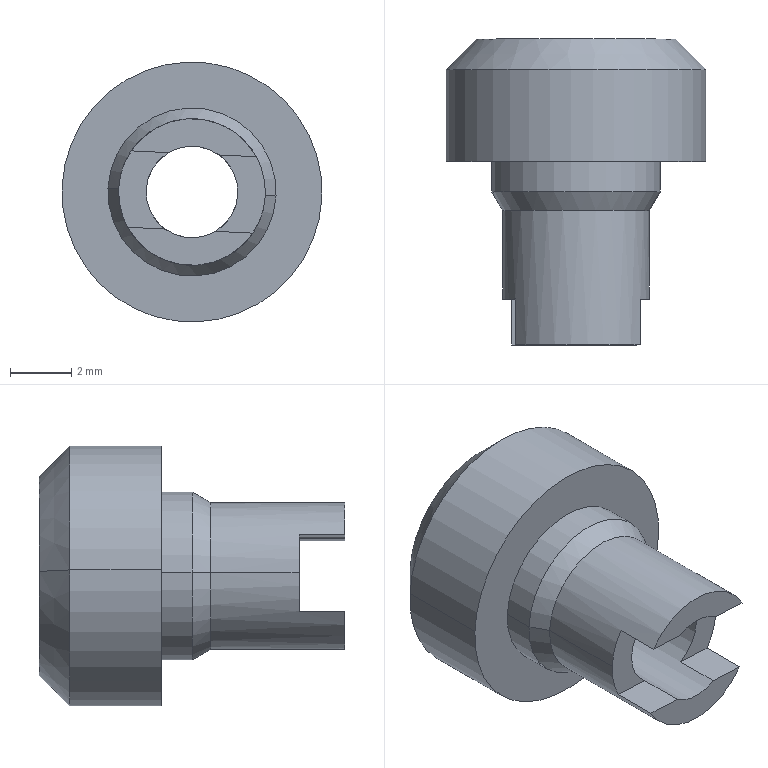Part | SolidWorks | features BaseBody 1 | 1 solid | 24 faces | box 8.5 x 10 x 8.5 mm | volume 252.316 mm3 | plane 10 | cylinder 8 | cone 6 | commonest cylinder face diameters 3 x2 4.8 x2 5.5 x2 8.5 x2
STEP:
#1=CARTESIAN_POINT('',(230.998,190.9,-0.07029));
#2=VERTEX_POINT('',#1);
#3=CARTESIAN_POINT('',(228.002,190.9,0.07029));
#4=VERTEX_POINT('',#3);
#5=CARTESIAN_POINT('',(229.5,190.9,0.));
#6=DIRECTION('',(0.,1.,0.));
#7=DIRECTION('',(0.9989,0.,-0.04686));
#8=AXIS2_PLACEMENT_3D('',#5,#6,#7);
#9=CIRCLE('',#8,1.5);
#10=EDGE_CURVE('',#2,#4,#9,.T.);
#11=ORIENTED_EDGE('',*,*,#10,.F.);
#12=CARTESIAN_POINT('',(231.198,191.1,-0.07966));
#13=VERTEX_POINT('',#12);
#14=CARTESIAN_POINT('',(230.998,190.9,-0.07029));
#15=DIRECTION('',(0.7063,0.7071,-0.03314));
#16=VECTOR('',#15,1000.);
#17=LINE('',#14,#16);
#18=EDGE_CURVE('',#2,#13,#17,.T.);
#19=ORIENTED_EDGE('',*,*,#18,.T.);
#20=CARTESIAN_POINT('',(227.802,191.1,0.07966));
#21=VERTEX_POINT('',#20);
#22=CARTESIAN_POINT('',(229.5,191.1,0.));
#23=DIRECTION('',(0.,-1.,0.));
#24=DIRECTION('',(0.9989,0.,-0.04686));
#25=AXIS2_PLACEMENT_3D('',#22,#23,#24);
#26=CIRCLE('',#25,1.7);
#27=EDGE_CURVE('',#21,#13,#26,.T.);
#28=ORIENTED_EDGE('',*,*,#27,.F.);
#29=CARTESIAN_POINT('',(228.002,190.9,0.07029));
#30=DIRECTION('',(-0.7063,0.7071,0.03314));
#31=VECTOR('',#30,1000.);
#32=LINE('',#29,#31);
#33=EDGE_CURVE('',#4,#21,#32,.T.);
#34=ORIENTED_EDGE('',*,*,#33,.F.);
#35=EDGE_LOOP('',(#11,#19,#28,#34));
#36=FACE_OUTER_BOUND('',#35,.T.);
#37=CARTESIAN_POINT('',(229.5,190.9,0.));
#38=DIRECTION('',(0.,1.,0.));
#39=DIRECTION('',(-0.9989,0.,0.04686));
#40=AXIS2_PLACEMENT_3D('',#37,#38,#39);
#41=CONICAL_SURFACE('',#40,1.5,0.7854);
#42=ADVANCED_FACE('',(#36),#41,.F.);
#43=CARTESIAN_POINT('',(226.254,191.1,0.1523));
#44=VERTEX_POINT('',#43);
#45=CARTESIAN_POINT('',(232.746,191.1,-0.1523));
#46=VERTEX_POINT('',#45);
#47=CARTESIAN_POINT('',(229.5,191.1,0.));
#48=DIRECTION('',(0.,1.,0.));
#49=DIRECTION('',(0.9989,0.,-0.04686));
#50=AXIS2_PLACEMENT_3D('',#47,#48,#49);
#51=CIRCLE('',#50,3.25);
#52=EDGE_CURVE('',#44,#46,#51,.T.);
#53=ORIENTED_EDGE('',*,*,#52,.F.);
#54=CARTESIAN_POINT('',(225.255,190.1,0.1992));
#55=VERTEX_POINT('',#54);
#56=CARTESIAN_POINT('',(226.254,191.1,0.1523));
#57=DIRECTION('',(-0.7063,-0.7071,0.03314));
#58=VECTOR('',#57,1000.);
#59=LINE('',#56,#58);
#60=EDGE_CURVE('',#44,#55,#59,.T.);
#61=ORIENTED_EDGE('',*,*,#60,.T.);
#62=CARTESIAN_POINT('',(233.745,190.1,-0.1992));
#63=VERTEX_POINT('',#62);
#64=CARTESIAN_POINT('',(229.5,190.1,0.));
#65=DIRECTION('',(0.,-1.,0.));
#66=DIRECTION('',(0.9989,0.,-0.04686));
#67=AXIS2_PLACEMENT_3D('',#64,#65,#66);
#68=CIRCLE('',#67,4.25);
#69=EDGE_CURVE('',#63,#55,#68,.T.);
#70=ORIENTED_EDGE('',*,*,#69,.F.);
#71=CARTESIAN_POINT('',(232.746,191.1,-0.1523));
#72=DIRECTION('',(0.7063,-0.7071,-0.03314));
#73=VECTOR('',#72,1000.);
#74=LINE('',#71,#73);
#75=EDGE_CURVE('',#46,#63,#74,.T.);
#76=ORIENTED_EDGE('',*,*,#75,.F.);
#77=EDGE_LOOP('',(#53,#61,#70,#76));
#78=FACE_OUTER_BOUND('',#77,.T.);
#79=CARTESIAN_POINT('',(229.5,191.1,0.));
#80=DIRECTION('',(0.,-1.,0.));
#81=DIRECTION('',(0.9989,0.,-0.04686));
#82=AXIS2_PLACEMENT_3D('',#79,#80,#81);
#83=CONICAL_SURFACE('',#82,3.25,0.7854);
#84=ADVANCED_FACE('',(#78),#83,.T.);
#85=CARTESIAN_POINT('',(227.103,185.494,0.1125));
#86=VERTEX_POINT('',#85);
#87=CARTESIAN_POINT('',(231.897,185.494,-0.1125));
#88=VERTEX_POINT('',#87);
#89=CARTESIAN_POINT('',(229.5,185.494,0.));
#90=DIRECTION('',(0.,1.,0.));
#91=DIRECTION('',(-0.9989,0.,0.04686));
#92=AXIS2_PLACEMENT_3D('',#89,#90,#91);
#93=CIRCLE('',#92,2.4);
#94=EDGE_CURVE('',#86,#88,#93,.T.);
#95=ORIENTED_EDGE('',*,*,#94,.T.);
#96=CARTESIAN_POINT('',(232.247,186.1,-0.1289));
#97=VERTEX_POINT('',#96);
#98=CARTESIAN_POINT('',(231.897,185.494,-0.1125));
#99=DIRECTION('',(0.4995,0.866,-0.02343));
#100=VECTOR('',#99,1000.);
#101=LINE('',#98,#100);
#102=EDGE_CURVE('',#88,#97,#101,.T.);
#103=ORIENTED_EDGE('',*,*,#102,.T.);
#104=CARTESIAN_POINT('',(226.753,186.1,0.1289));
#105=VERTEX_POINT('',#104);
#106=CARTESIAN_POINT('',(229.5,186.1,0.));
#107=DIRECTION('',(0.,1.,0.));
#108=DIRECTION('',(-0.9989,0.,0.04686));
#109=AXIS2_PLACEMENT_3D('',#106,#107,#108);
#110=CIRCLE('',#109,2.75);
#111=EDGE_CURVE('',#105,#97,#110,.T.);
#112=ORIENTED_EDGE('',*,*,#111,.F.);
#113=CARTESIAN_POINT('',(227.103,185.494,0.1125));
#114=DIRECTION('',(-0.4995,0.866,0.02343));
#115=VECTOR('',#114,1000.);
#116=LINE('',#113,#115);
#117=EDGE_CURVE('',#86,#105,#116,.T.);
#118=ORIENTED_EDGE('',*,*,#117,.F.);
#119=EDGE_LOOP('',(#95,#103,#112,#118));
#120=FACE_OUTER_BOUND('',#119,.T.);
#121=CARTESIAN_POINT('',(229.5,185.494,0.));
#122=DIRECTION('',(0.,1.,0.));
#123=DIRECTION('',(-0.9989,0.,0.04686));
#124=AXIS2_PLACEMENT_3D('',#121,#122,#123);
#125=CONICAL_SURFACE('',#124,2.4,0.5236);
#126=ADVANCED_FACE('',(#120),#125,.T.);
#127=ORIENTED_EDGE('',*,*,#111,.T.);
#128=CARTESIAN_POINT('',(232.247,187.1,-0.1289));
#129=VERTEX_POINT('',#128);
#130=CARTESIAN_POINT('',(232.247,192.536,-0.1289));
#131=DIRECTION('',(0.,1.,0.));
#132=VECTOR('',#131,1000.);
#133=LINE('',#130,#132);
#134=EDGE_CURVE('',#97,#129,#133,.T.);
#135=ORIENTED_EDGE('',*,*,#134,.T.);
#136=CARTESIAN_POINT('',(226.753,187.1,0.1289));
#137=VERTEX_POINT('',#136);
#138=CARTESIAN_POINT('',(229.5,187.1,0.));
#139=DIRECTION('',(0.,1.,0.));
#140=DIRECTION('',(-0.9989,0.,0.04686));
#141=AXIS2_PLACEMENT_3D('',#138,#139,#140);
#142=CIRCLE('',#141,2.75);
#143=EDGE_CURVE('',#137,#129,#142,.T.);
#144=ORIENTED_EDGE('',*,*,#143,.F.);
#145=CARTESIAN_POINT('',(226.753,192.536,0.1289));
#146=DIRECTION('',(0.,1.,0.));
#147=VECTOR('',#146,1000.);
#148=LINE('',#145,#147);
#149=EDGE_CURVE('',#105,#137,#148,.T.);
#150=ORIENTED_EDGE('',*,*,#149,.F.);
#151=EDGE_LOOP('',(#127,#135,#144,#150));
#152=FACE_OUTER_BOUND('',#151,.T.);
#153=CARTESIAN_POINT('',(229.5,192.536,0.));
#154=DIRECTION('',(0.,1.,0.));
#155=DIRECTION('',(-0.9989,0.,0.04686));
#156=AXIS2_PLACEMENT_3D('',#153,#154,#155);
#157=CYLINDRICAL_SURFACE('',#156,2.75);
#158=ADVANCED_FACE('',(#152),#157,.T.);
#159=CARTESIAN_POINT('',(225.255,187.1,0.1992));
#160=VERTEX_POINT('',#159);
#161=CARTESIAN_POINT('',(233.745,187.1,-0.1992));
#162=VERTEX_POINT('',#161);
#163=CARTESIAN_POINT('',(229.5,187.1,0.));
#164=DIRECTION('',(0.,1.,0.));
#165=DIRECTION('',(-0.9989,0.,0.04686));
#166=AXIS2_PLACEMENT_3D('',#163,#164,#165);
#167=CIRCLE('',#166,4.25);
#168=EDGE_CURVE('',#160,#162,#167,.T.);
#169=ORIENTED_EDGE('',*,*,#168,.T.);
#170=CARTESIAN_POINT('',(233.745,192.536,-0.1992));
#171=DIRECTION('',(0.,1.,0.));
#172=VECTOR('',#171,1000.);
#173=LINE('',#170,#172);
#174=EDGE_CURVE('',#162,#63,#173,.T.);
#175=ORIENTED_EDGE('',*,*,#174,.T.);
#176=ORIENTED_EDGE('',*,*,#69,.T.);
#177=CARTESIAN_POINT('',(225.255,192.536,0.1992));
#178=DIRECTION('',(0.,1.,0.));
#179=VECTOR('',#178,1000.);
#180=LINE('',#177,#179);
#181=EDGE_CURVE('',#160,#55,#180,.T.);
#182=ORIENTED_EDGE('',*,*,#181,.F.);
#183=EDGE_LOOP('',(#169,#175,#176,#182));
#184=FACE_OUTER_BOUND('',#183,.T.);
#185=CARTESIAN_POINT('',(229.5,192.536,0.));
#186=DIRECTION('',(0.,1.,0.));
#187=DIRECTION('',(-0.9989,0.,0.04686));
#188=AXIS2_PLACEMENT_3D('',#185,#186,#187);
#189=CYLINDRICAL_SURFACE('',#188,4.25);
#190=ADVANCED_FACE('',(#184),#189,.T.);
#191=CARTESIAN_POINT('',(230.27,182.6,-1.287));
#192=VERTEX_POINT('',#191);
#193=CARTESIAN_POINT('',(230.998,182.6,-0.07029));
#194=VERTEX_POINT('',#193);
#195=CARTESIAN_POINT('',(229.5,182.6,0.));
#196=DIRECTION('',(0.,-1.,0.));
#197=DIRECTION('',(0.9989,0.,-0.04686));
#198=AXIS2_PLACEMENT_3D('',#195,#196,#197);
#199=CIRCLE('',#198,1.5);
#200=EDGE_CURVE('',#192,#194,#199,.T.);
#201=ORIENTED_EDGE('',*,*,#200,.T.);
#202=CARTESIAN_POINT('',(230.998,192.536,-0.07029));
#203=DIRECTION('',(0.,1.,0.));
#204=VECTOR('',#203,1000.);
#205=LINE('',#202,#204);
#206=EDGE_CURVE('',#194,#2,#205,.T.);
#207=ORIENTED_EDGE('',*,*,#206,.T.);
#208=ORIENTED_EDGE('',*,*,#10,.T.);
#209=CARTESIAN_POINT('',(228.002,182.6,0.07029));
#210=VERTEX_POINT('',#209);
#211=CARTESIAN_POINT('',(228.002,192.536,0.07029));
#212=DIRECTION('',(0.,1.,0.));
#213=VECTOR('',#212,1000.);
#214=LINE('',#211,#213);
#215=EDGE_CURVE('',#210,#4,#214,.T.);
#216=ORIENTED_EDGE('',*,*,#215,.F.);
#217=CARTESIAN_POINT('',(228.613,182.6,-1.21));
#218=VERTEX_POINT('',#217);
#219=CARTESIAN_POINT('',(229.5,182.6,0.));
#220=DIRECTION('',(0.,1.,0.));
#221=DIRECTION('',(-0.9989,0.,0.04686));
#222=AXIS2_PLACEMENT_3D('',#219,#220,#221);
#223=CIRCLE('',#222,1.5);
#224=EDGE_CURVE('',#218,#210,#223,.T.);
#225=ORIENTED_EDGE('',*,*,#224,.F.);
#226=CARTESIAN_POINT('',(228.613,181.1,-1.21));
#227=VERTEX_POINT('',#226);
#228=CARTESIAN_POINT('',(228.613,192.536,-1.21));
#229=DIRECTION('',(0.,1.,0.));
#230=VECTOR('',#229,1000.);
#231=LINE('',#228,#230);
#232=EDGE_CURVE('',#227,#218,#231,.T.);
#233=ORIENTED_EDGE('',*,*,#232,.F.);
#234=CARTESIAN_POINT('',(230.27,181.1,-1.287));
#235=VERTEX_POINT('',#234);
#236=CARTESIAN_POINT('',(229.5,181.1,0.));
#237=DIRECTION('',(0.,1.,0.));
#238=DIRECTION('',(-0.9989,0.,0.04686));
#239=AXIS2_PLACEMENT_3D('',#236,#237,#238);
#240=CIRCLE('',#239,1.5);
#241=EDGE_CURVE('',#235,#227,#240,.T.);
#242=ORIENTED_EDGE('',*,*,#241,.F.);
#243=CARTESIAN_POINT('',(230.27,192.536,-1.287));
#244=DIRECTION('',(0.,1.,0.));
#245=VECTOR('',#244,1000.);
#246=LINE('',#243,#245);
#247=EDGE_CURVE('',#235,#192,#246,.T.);
#248=ORIENTED_EDGE('',*,*,#247,.T.);
#249=EDGE_LOOP('',(#201,#207,#208,#216,#225,#233,#242,#248));
#250=FACE_OUTER_BOUND('',#249,.T.);
#251=CARTESIAN_POINT('',(229.5,192.536,0.));
#252=DIRECTION('',(0.,1.,0.));
#253=DIRECTION('',(-0.9989,0.,0.04686));
#254=AXIS2_PLACEMENT_3D('',#251,#252,#253);
#255=CYLINDRICAL_SURFACE('',#254,1.5);
#256=ADVANCED_FACE('',(#250),#255,.F.);
#257=CARTESIAN_POINT('',(231.605,182.6,1.153));
#258=VERTEX_POINT('',#257);
#259=CARTESIAN_POINT('',(231.897,182.6,-0.1125));
#260=VERTEX_POINT('',#259);
#261=CARTESIAN_POINT('',(229.5,182.6,0.));
#262=DIRECTION('',(0.,1.,0.));
#263=DIRECTION('',(0.9989,0.,-0.04686));
#264=AXIS2_PLACEMENT_3D('',#261,#262,#263);
#265=CIRCLE('',#264,2.4);
#266=EDGE_CURVE('',#258,#260,#265,.T.);
#267=ORIENTED_EDGE('',*,*,#266,.T.);
#268=CARTESIAN_POINT('',(231.897,192.536,-0.1125));
#269=DIRECTION('',(0.,1.,0.));
#270=VECTOR('',#269,1000.);
#271=LINE('',#268,#270);
#272=EDGE_CURVE('',#260,#88,#271,.T.);
#273=ORIENTED_EDGE('',*,*,#272,.T.);
#274=ORIENTED_EDGE('',*,*,#94,.F.);
#275=CARTESIAN_POINT('',(227.103,182.6,0.1125));
#276=VERTEX_POINT('',#275);
#277=CARTESIAN_POINT('',(227.103,192.536,0.1125));
#278=DIRECTION('',(0.,1.,0.));
#279=VECTOR('',#278,1000.);
#280=LINE('',#277,#279);
#281=EDGE_CURVE('',#276,#86,#280,.T.);
#282=ORIENTED_EDGE('',*,*,#281,.F.);
#283=CARTESIAN_POINT('',(227.512,182.6,1.345));
#284=VERTEX_POINT('',#283);
#285=CARTESIAN_POINT('',(229.5,182.6,0.));
#286=DIRECTION('',(0.,-1.,0.));
#287=DIRECTION('',(-0.9989,0.,0.04686));
#288=AXIS2_PLACEMENT_3D('',#285,#286,#287);
#289=CIRCLE('',#288,2.4);
#290=EDGE_CURVE('',#284,#276,#289,.T.);
#291=ORIENTED_EDGE('',*,*,#290,.F.);
#292=CARTESIAN_POINT('',(227.512,181.1,1.345));
#293=VERTEX_POINT('',#292);
#294=CARTESIAN_POINT('',(227.512,192.536,1.345));
#295=DIRECTION('',(0.,1.,0.));
#296=VECTOR('',#295,1000.);
#297=LINE('',#294,#296);
#298=EDGE_CURVE('',#293,#284,#297,.T.);
#299=ORIENTED_EDGE('',*,*,#298,.F.);
#300=CARTESIAN_POINT('',(231.605,181.1,1.153));
#301=VERTEX_POINT('',#300);
#302=CARTESIAN_POINT('',(229.5,181.1,0.));
#303=DIRECTION('',(0.,1.,0.));
#304=DIRECTION('',(-0.9989,0.,0.04686));
#305=AXIS2_PLACEMENT_3D('',#302,#303,#304);
#306=CIRCLE('',#305,2.4);
#307=EDGE_CURVE('',#293,#301,#306,.T.);
#308=ORIENTED_EDGE('',*,*,#307,.T.);
#309=CARTESIAN_POINT('',(231.605,192.536,1.153));
#310=DIRECTION('',(0.,1.,0.));
#311=VECTOR('',#310,1000.);
#312=LINE('',#309,#311);
#313=EDGE_CURVE('',#301,#258,#312,.T.);
#314=ORIENTED_EDGE('',*,*,#313,.T.);
#315=EDGE_LOOP('',(#267,#273,#274,#282,#291,#299,#308,#314));
#316=FACE_OUTER_BOUND('',#315,.T.);
#317=CARTESIAN_POINT('',(229.5,192.536,0.));
#318=DIRECTION('',(0.,1.,0.));
#319=DIRECTION('',(-0.9989,0.,0.04686));
#320=AXIS2_PLACEMENT_3D('',#317,#318,#319);
#321=CYLINDRICAL_SURFACE('',#320,2.4);
#322=ADVANCED_FACE('',(#316),#321,.T.);
#323=ORIENTED_EDGE('',*,*,#307,.F.);
#324=CARTESIAN_POINT('',(228.73,181.1,1.287));
#325=VERTEX_POINT('',#324);
#326=CARTESIAN_POINT('',(225.312,181.1,1.448));
#327=DIRECTION('',(0.9989,0.,-0.04686));
#328=VECTOR('',#327,1000.);
#329=LINE('',#326,#328);
#330=EDGE_CURVE('',#293,#325,#329,.T.);
#331=ORIENTED_EDGE('',*,*,#330,.T.);
#332=CARTESIAN_POINT('',(230.387,181.1,1.21));
#333=VERTEX_POINT('',#332);
#334=CARTESIAN_POINT('',(229.5,181.1,0.));
#335=DIRECTION('',(0.,1.,0.));
#336=DIRECTION('',(-0.9989,0.,0.04686));
#337=AXIS2_PLACEMENT_3D('',#334,#335,#336);
#338=CIRCLE('',#337,1.5);
#339=EDGE_CURVE('',#325,#333,#338,.T.);
#340=ORIENTED_EDGE('',*,*,#339,.T.);
#341=CARTESIAN_POINT('',(233.805,181.1,1.049));
#342=DIRECTION('',(-0.9989,0.,0.04686));
#343=VECTOR('',#342,1000.);
#344=LINE('',#341,#343);
#345=EDGE_CURVE('',#301,#333,#344,.T.);
#346=ORIENTED_EDGE('',*,*,#345,.F.);
#347=EDGE_LOOP('',(#323,#331,#340,#346));
#348=FACE_OUTER_BOUND('',#347,.T.);
#349=CARTESIAN_POINT('',(229.388,181.1,-2.397));
#350=DIRECTION('',(0.,1.,0.));
#351=DIRECTION('',(-0.9989,0.,0.04686));
#352=AXIS2_PLACEMENT_3D('',#349,#350,#351);
#353=PLANE('',#352);
#354=ADVANCED_FACE('',(#348),#353,.F.);
#355=ORIENTED_EDGE('',*,*,#272,.F.);
#356=CARTESIAN_POINT('',(231.488,182.6,-1.345));
#357=VERTEX_POINT('',#356);
#358=CARTESIAN_POINT('',(229.5,182.6,0.));
#359=DIRECTION('',(0.,1.,0.));
#360=DIRECTION('',(0.9989,0.,-0.04686));
#361=AXIS2_PLACEMENT_3D('',#358,#359,#360);
#362=CIRCLE('',#361,2.4);
#363=EDGE_CURVE('',#260,#357,#362,.T.);
#364=ORIENTED_EDGE('',*,*,#363,.T.);
#365=CARTESIAN_POINT('',(231.488,181.1,-1.345));
#366=VERTEX_POINT('',#365);
#367=CARTESIAN_POINT('',(231.488,192.536,-1.345));
#368=DIRECTION('',(0.,-1.,0.));
#369=VECTOR('',#368,1000.);
#370=LINE('',#367,#369);
#371=EDGE_CURVE('',#357,#366,#370,.T.);
#372=ORIENTED_EDGE('',*,*,#371,.T.);
#373=CARTESIAN_POINT('',(227.395,181.1,-1.153));
#374=VERTEX_POINT('',#373);
#375=CARTESIAN_POINT('',(229.5,181.1,0.));
#376=DIRECTION('',(0.,1.,0.));
#377=DIRECTION('',(-0.9989,0.,0.04686));
#378=AXIS2_PLACEMENT_3D('',#375,#376,#377);
#379=CIRCLE('',#378,2.4);
#380=EDGE_CURVE('',#366,#374,#379,.T.);
#381=ORIENTED_EDGE('',*,*,#380,.T.);
#382=CARTESIAN_POINT('',(227.395,182.6,-1.153));
#383=VERTEX_POINT('',#382);
#384=CARTESIAN_POINT('',(227.395,192.536,-1.153));
#385=DIRECTION('',(0.,-1.,0.));
#386=VECTOR('',#385,1000.);
#387=LINE('',#384,#386);
#388=EDGE_CURVE('',#383,#374,#387,.T.);
#389=ORIENTED_EDGE('',*,*,#388,.F.);
#390=CARTESIAN_POINT('',(229.5,182.6,0.));
#391=DIRECTION('',(0.,-1.,0.));
#392=DIRECTION('',(-0.9989,0.,0.04686));
#393=AXIS2_PLACEMENT_3D('',#390,#391,#392);
#394=CIRCLE('',#393,2.4);
#395=EDGE_CURVE('',#276,#383,#394,.T.);
#396=ORIENTED_EDGE('',*,*,#395,.F.);
#397=ORIENTED_EDGE('',*,*,#281,.T.);
#398=CARTESIAN_POINT('',(229.5,185.494,0.));
#399=DIRECTION('',(0.,1.,0.));
#400=DIRECTION('',(-0.9989,0.,0.04686));
#401=AXIS2_PLACEMENT_3D('',#398,#399,#400);
#402=CIRCLE('',#401,2.4);
#403=EDGE_CURVE('',#88,#86,#402,.T.);
#404=ORIENTED_EDGE('',*,*,#403,.F.);
#405=EDGE_LOOP('',(#355,#364,#372,#381,#389,#396,#397,#404));
#406=FACE_OUTER_BOUND('',#405,.T.);
#407=CARTESIAN_POINT('',(229.5,192.536,0.));
#408=DIRECTION('',(0.,1.,0.));
#409=DIRECTION('',(-0.9989,0.,0.04686));
#410=AXIS2_PLACEMENT_3D('',#407,#408,#409);
#411=CYLINDRICAL_SURFACE('',#410,2.4);
#412=ADVANCED_FACE('',(#406),#411,.T.);
#413=ORIENTED_EDGE('',*,*,#241,.T.);
#414=CARTESIAN_POINT('',(225.195,181.1,-1.049));
#415=DIRECTION('',(0.9989,0.,-0.04686));
#416=VECTOR('',#415,1000.);
#417=LINE('',#414,#416);
#418=EDGE_CURVE('',#374,#227,#417,.T.);
#419=ORIENTED_EDGE('',*,*,#418,.F.);
#420=ORIENTED_EDGE('',*,*,#380,.F.);
#421=CARTESIAN_POINT('',(233.688,181.1,-1.448));
#422=DIRECTION('',(-0.9989,0.,0.04686));
#423=VECTOR('',#422,1000.);
#424=LINE('',#421,#423);
#425=EDGE_CURVE('',#366,#235,#424,.T.);
#426=ORIENTED_EDGE('',*,*,#425,.T.);
#427=EDGE_LOOP('',(#413,#419,#420,#426));
#428=FACE_OUTER_BOUND('',#427,.T.);
#429=CARTESIAN_POINT('',(229.388,181.1,-2.397));
#430=DIRECTION('',(0.,1.,0.));
#431=DIRECTION('',(-0.9989,0.,0.04686));
#432=AXIS2_PLACEMENT_3D('',#429,#430,#431);
#433=PLANE('',#432);
#434=ADVANCED_FACE('',(#428),#433,.F.);
#435=ORIENTED_EDGE('',*,*,#206,.F.);
#436=CARTESIAN_POINT('',(230.387,182.6,1.21));
#437=VERTEX_POINT('',#436);
#438=CARTESIAN_POINT('',(229.5,182.6,0.));
#439=DIRECTION('',(0.,-1.,0.));
#440=DIRECTION('',(0.9989,0.,-0.04686));
#441=AXIS2_PLACEMENT_3D('',#438,#439,#440);
#442=CIRCLE('',#441,1.5);
#443=EDGE_CURVE('',#194,#437,#442,.T.);
#444=ORIENTED_EDGE('',*,*,#443,.T.);
#445=CARTESIAN_POINT('',(230.387,192.536,1.21));
#446=DIRECTION('',(0.,-1.,0.));
#447=VECTOR('',#446,1000.);
#448=LINE('',#445,#447);
#449=EDGE_CURVE('',#437,#333,#448,.T.);
#450=ORIENTED_EDGE('',*,*,#449,.T.);
#451=ORIENTED_EDGE('',*,*,#339,.F.);
#452=CARTESIAN_POINT('',(228.73,182.6,1.287));
#453=VERTEX_POINT('',#452);
#454=CARTESIAN_POINT('',(228.73,192.536,1.287));
#455=DIRECTION('',(0.,-1.,0.));
#456=VECTOR('',#455,1000.);
#457=LINE('',#454,#456);
#458=EDGE_CURVE('',#453,#325,#457,.T.);
#459=ORIENTED_EDGE('',*,*,#458,.F.);
#460=CARTESIAN_POINT('',(229.5,182.6,0.));
#461=DIRECTION('',(0.,1.,0.));
#462=DIRECTION('',(-0.9989,0.,0.04686));
#463=AXIS2_PLACEMENT_3D('',#460,#461,#462);
#464=CIRCLE('',#463,1.5);
#465=EDGE_CURVE('',#210,#453,#464,.T.);
#466=ORIENTED_EDGE('',*,*,#465,.F.);
#467=ORIENTED_EDGE('',*,*,#215,.T.);
#468=CARTESIAN_POINT('',(229.5,190.9,0.));
#469=DIRECTION('',(0.,1.,0.));
#470=DIRECTION('',(0.9989,0.,-0.04686));
#471=AXIS2_PLACEMENT_3D('',#468,#469,#470);
#472=CIRCLE('',#471,1.5);
#473=EDGE_CURVE('',#4,#2,#472,.T.);
#474=ORIENTED_EDGE('',*,*,#473,.T.);
#475=EDGE_LOOP('',(#435,#444,#450,#451,#459,#466,#467,#474));
#476=FACE_OUTER_BOUND('',#475,.T.);
#477=CARTESIAN_POINT('',(229.5,192.536,0.));
#478=DIRECTION('',(0.,1.,0.));
#479=DIRECTION('',(-0.9989,0.,0.04686));
#480=AXIS2_PLACEMENT_3D('',#477,#478,#479);
#481=CYLINDRICAL_SURFACE('',#480,1.5);
#482=ADVANCED_FACE('',(#476),#481,.F.);
#483=ORIENTED_EDGE('',*,*,#174,.F.);
#484=CARTESIAN_POINT('',(229.5,187.1,0.));
#485=DIRECTION('',(0.,1.,0.));
#486=DIRECTION('',(-0.9989,0.,0.04686));
#487=AXIS2_PLACEMENT_3D('',#484,#485,#486);
#488=CIRCLE('',#487,4.25);
#489=EDGE_CURVE('',#162,#160,#488,.T.);
#490=ORIENTED_EDGE('',*,*,#489,.T.);
#491=ORIENTED_EDGE('',*,*,#181,.T.);
#492=CARTESIAN_POINT('',(229.5,190.1,0.));
#493=DIRECTION('',(0.,-1.,0.));
#494=DIRECTION('',(0.9989,0.,-0.04686));
#495=AXIS2_PLACEMENT_3D('',#492,#493,#494);
#496=CIRCLE('',#495,4.25);
#497=EDGE_CURVE('',#55,#63,#496,.T.);
#498=ORIENTED_EDGE('',*,*,#497,.T.);
#499=EDGE_LOOP('',(#483,#490,#491,#498));
#500=FACE_OUTER_BOUND('',#499,.T.);
#501=CARTESIAN_POINT('',(229.5,192.536,0.));
#502=DIRECTION('',(0.,1.,0.));
#503=DIRECTION('',(-0.9989,0.,0.04686));
#504=AXIS2_PLACEMENT_3D('',#501,#502,#503);
#505=CYLINDRICAL_SURFACE('',#504,4.25);
#506=ADVANCED_FACE('',(#500),#505,.T.);
#507=ORIENTED_EDGE('',*,*,#168,.F.);
#508=ORIENTED_EDGE('',*,*,#489,.F.);
#509=EDGE_LOOP('',(#507,#508));
#510=FACE_OUTER_BOUND('',#509,.T.);
#511=ORIENTED_EDGE('',*,*,#143,.T.);
#512=CARTESIAN_POINT('',(229.5,187.1,0.));
#513=DIRECTION('',(0.,1.,0.));
#514=DIRECTION('',(-0.9989,0.,0.04686));
#515=AXIS2_PLACEMENT_3D('',#512,#513,#514);
#516=CIRCLE('',#515,2.75);
#517=EDGE_CURVE('',#129,#137,#516,.T.);
#518=ORIENTED_EDGE('',*,*,#517,.T.);
#519=EDGE_LOOP('',(#511,#518));
#520=FACE_BOUND('',#519,.T.);
#521=CARTESIAN_POINT('',(229.301,187.1,-4.245));
#522=DIRECTION('',(0.,1.,0.));
#523=DIRECTION('',(-0.9989,0.,0.04686));
#524=AXIS2_PLACEMENT_3D('',#521,#522,#523);
#525=PLANE('',#524);
#526=ADVANCED_FACE('',(#510,#520),#525,.F.);
#527=ORIENTED_EDGE('',*,*,#134,.F.);
#528=CARTESIAN_POINT('',(229.5,186.1,0.));
#529=DIRECTION('',(0.,1.,0.));
#530=DIRECTION('',(-0.9989,0.,0.04686));
#531=AXIS2_PLACEMENT_3D('',#528,#529,#530);
#532=CIRCLE('',#531,2.75);
#533=EDGE_CURVE('',#97,#105,#532,.T.);
#534=ORIENTED_EDGE('',*,*,#533,.T.);
#535=ORIENTED_EDGE('',*,*,#149,.T.);
#536=ORIENTED_EDGE('',*,*,#517,.F.);
#537=EDGE_LOOP('',(#527,#534,#535,#536));
#538=FACE_OUTER_BOUND('',#537,.T.);
#539=CARTESIAN_POINT('',(229.5,192.536,0.));
#540=DIRECTION('',(0.,1.,0.));
#541=DIRECTION('',(-0.9989,0.,0.04686));
#542=AXIS2_PLACEMENT_3D('',#539,#540,#541);
#543=CYLINDRICAL_SURFACE('',#542,2.75);
#544=ADVANCED_FACE('',(#538),#543,.T.);
#545=ORIENTED_EDGE('',*,*,#102,.F.);
#546=ORIENTED_EDGE('',*,*,#403,.T.);
#547=ORIENTED_EDGE('',*,*,#117,.T.);
#548=ORIENTED_EDGE('',*,*,#533,.F.);
#549=EDGE_LOOP('',(#545,#546,#547,#548));
#550=FACE_OUTER_BOUND('',#549,.T.);
#551=CARTESIAN_POINT('',(229.5,185.494,0.));
#552=DIRECTION('',(0.,1.,0.));
#553=DIRECTION('',(-0.9989,0.,0.04686));
#554=AXIS2_PLACEMENT_3D('',#551,#552,#553);
#555=CONICAL_SURFACE('',#554,2.4,0.5236);
#556=ADVANCED_FACE('',(#550),#555,.T.);
#557=ORIENTED_EDGE('',*,*,#27,.T.);
#558=CARTESIAN_POINT('',(229.5,191.1,0.));
#559=DIRECTION('',(0.,-1.,0.));
#560=DIRECTION('',(0.9989,0.,-0.04686));
#561=AXIS2_PLACEMENT_3D('',#558,#559,#560);
#562=CIRCLE('',#561,1.7);
#563=EDGE_CURVE('',#13,#21,#562,.T.);
#564=ORIENTED_EDGE('',*,*,#563,.T.);
#565=EDGE_LOOP('',(#557,#564));
#566=FACE_BOUND('',#565,.T.);
#567=CARTESIAN_POINT('',(229.5,191.1,0.));
#568=DIRECTION('',(0.,1.,0.));
#569=DIRECTION('',(0.9989,0.,-0.04686));
#570=AXIS2_PLACEMENT_3D('',#567,#568,#569);
#571=CIRCLE('',#570,3.25);
#572=EDGE_CURVE('',#46,#44,#571,.T.);
#573=ORIENTED_EDGE('',*,*,#572,.T.);
#574=ORIENTED_EDGE('',*,*,#52,.T.);
#575=EDGE_LOOP('',(#573,#574));
#576=FACE_OUTER_BOUND('',#575,.T.);
#577=CARTESIAN_POINT('',(229.43,191.1,-1.498));
#578=DIRECTION('',(0.,-1.,0.));
#579=DIRECTION('',(0.9989,0.,-0.04686));
#580=AXIS2_PLACEMENT_3D('',#577,#578,#579);
#581=PLANE('',#580);
#582=ADVANCED_FACE('',(#566,#576),#581,.F.);
#583=ORIENTED_EDGE('',*,*,#60,.F.);
#584=ORIENTED_EDGE('',*,*,#572,.F.);
#585=ORIENTED_EDGE('',*,*,#75,.T.);
#586=ORIENTED_EDGE('',*,*,#497,.F.);
#587=EDGE_LOOP('',(#583,#584,#585,#586));
#588=FACE_OUTER_BOUND('',#587,.T.);
#589=CARTESIAN_POINT('',(229.5,191.1,0.));
#590=DIRECTION('',(0.,-1.,0.));
#591=DIRECTION('',(0.9989,0.,-0.04686));
#592=AXIS2_PLACEMENT_3D('',#589,#590,#591);
#593=CONICAL_SURFACE('',#592,3.25,0.7854);
#594=ADVANCED_FACE('',(#588),#593,.T.);
#595=ORIENTED_EDGE('',*,*,#18,.F.);
#596=ORIENTED_EDGE('',*,*,#473,.F.);
#597=ORIENTED_EDGE('',*,*,#33,.T.);
#598=ORIENTED_EDGE('',*,*,#563,.F.);
#599=EDGE_LOOP('',(#595,#596,#597,#598));
#600=FACE_OUTER_BOUND('',#599,.T.);
#601=CARTESIAN_POINT('',(229.5,190.9,0.));
#602=DIRECTION('',(0.,1.,0.));
#603=DIRECTION('',(-0.9989,0.,0.04686));
#604=AXIS2_PLACEMENT_3D('',#601,#602,#603);
#605=CONICAL_SURFACE('',#604,1.5,0.7854);
#606=ADVANCED_FACE('',(#600),#605,.F.);
#607=CARTESIAN_POINT('',(233.688,182.6,-1.448));
#608=DIRECTION('',(-0.9989,0.,0.04686));
#609=VECTOR('',#608,1000.);
#610=LINE('',#607,#609);
#611=EDGE_CURVE('',#357,#192,#610,.T.);
#612=ORIENTED_EDGE('',*,*,#611,.T.);
#613=ORIENTED_EDGE('',*,*,#247,.F.);
#614=ORIENTED_EDGE('',*,*,#425,.F.);
#615=ORIENTED_EDGE('',*,*,#371,.F.);
#616=EDGE_LOOP('',(#612,#613,#614,#615));
#617=FACE_OUTER_BOUND('',#616,.T.);
#618=CARTESIAN_POINT('',(233.688,181.1,-1.448));
#619=DIRECTION('',(0.04686,0.,0.9989));
#620=DIRECTION('',(0.,-1.,0.));
#621=AXIS2_PLACEMENT_3D('',#618,#619,#620);
#622=PLANE('',#621);
#623=ADVANCED_FACE('',(#617),#622,.T.);
#624=CARTESIAN_POINT('',(233.805,182.6,1.049));
#625=DIRECTION('',(-0.9989,0.,0.04686));
#626=VECTOR('',#625,1000.);
#627=LINE('',#624,#626);
#628=EDGE_CURVE('',#258,#437,#627,.T.);
#629=ORIENTED_EDGE('',*,*,#628,.T.);
#630=ORIENTED_EDGE('',*,*,#443,.F.);
#631=ORIENTED_EDGE('',*,*,#200,.F.);
#632=ORIENTED_EDGE('',*,*,#611,.F.);
#633=ORIENTED_EDGE('',*,*,#363,.F.);
#634=ORIENTED_EDGE('',*,*,#266,.F.);
#635=EDGE_LOOP('',(#629,#630,#631,#632,#633,#634));
#636=FACE_OUTER_BOUND('',#635,.T.);
#637=CARTESIAN_POINT('',(233.688,182.6,-1.448));
#638=DIRECTION('',(0.,-1.,0.));
#639=DIRECTION('',(0.9989,0.,-0.04686));
#640=AXIS2_PLACEMENT_3D('',#637,#638,#639);
#641=PLANE('',#640);
#642=ADVANCED_FACE('',(#636),#641,.T.);
#643=ORIENTED_EDGE('',*,*,#345,.T.);
#644=ORIENTED_EDGE('',*,*,#449,.F.);
#645=ORIENTED_EDGE('',*,*,#628,.F.);
#646=ORIENTED_EDGE('',*,*,#313,.F.);
#647=EDGE_LOOP('',(#643,#644,#645,#646));
#648=FACE_OUTER_BOUND('',#647,.T.);
#649=CARTESIAN_POINT('',(233.805,182.6,1.049));
#650=DIRECTION('',(-0.04686,0.,-0.9989));
#651=DIRECTION('',(0.,1.,0.));
#652=AXIS2_PLACEMENT_3D('',#649,#650,#651);
#653=PLANE('',#652);
#654=ADVANCED_FACE('',(#648),#653,.T.);
#655=ORIENTED_EDGE('',*,*,#298,.T.);
#656=CARTESIAN_POINT('',(225.312,182.6,1.448));
#657=DIRECTION('',(0.9989,0.,-0.04686));
#658=VECTOR('',#657,1000.);
#659=LINE('',#656,#658);
#660=EDGE_CURVE('',#284,#453,#659,.T.);
#661=ORIENTED_EDGE('',*,*,#660,.T.);
#662=ORIENTED_EDGE('',*,*,#458,.T.);
#663=ORIENTED_EDGE('',*,*,#330,.F.);
#664=EDGE_LOOP('',(#655,#661,#662,#663));
#665=FACE_OUTER_BOUND('',#664,.T.);
#666=CARTESIAN_POINT('',(225.312,182.6,1.448));
#667=DIRECTION('',(0.04686,0.,0.9989));
#668=DIRECTION('',(0.,-1.,0.));
#669=AXIS2_PLACEMENT_3D('',#666,#667,#668);
#670=PLANE('',#669);
#671=ADVANCED_FACE('',(#665),#670,.F.);
#672=ORIENTED_EDGE('',*,*,#290,.T.);
#673=ORIENTED_EDGE('',*,*,#395,.T.);
#674=CARTESIAN_POINT('',(225.195,182.6,-1.049));
#675=DIRECTION('',(0.9989,0.,-0.04686));
#676=VECTOR('',#675,1000.);
#677=LINE('',#674,#676);
#678=EDGE_CURVE('',#383,#218,#677,.T.);
#679=ORIENTED_EDGE('',*,*,#678,.T.);
#680=ORIENTED_EDGE('',*,*,#224,.T.);
#681=ORIENTED_EDGE('',*,*,#465,.T.);
#682=ORIENTED_EDGE('',*,*,#660,.F.);
#683=EDGE_LOOP('',(#672,#673,#679,#680,#681,#682));
#684=FACE_OUTER_BOUND('',#683,.T.);
#685=CARTESIAN_POINT('',(225.195,182.6,-1.049));
#686=DIRECTION('',(0.,1.,0.));
#687=DIRECTION('',(-0.9989,0.,0.04686));
#688=AXIS2_PLACEMENT_3D('',#685,#686,#687);
#689=PLANE('',#688);
#690=ADVANCED_FACE('',(#684),#689,.F.);
#691=ORIENTED_EDGE('',*,*,#388,.T.);
#692=ORIENTED_EDGE('',*,*,#418,.T.);
#693=ORIENTED_EDGE('',*,*,#232,.T.);
#694=ORIENTED_EDGE('',*,*,#678,.F.);
#695=EDGE_LOOP('',(#691,#692,#693,#694));
#696=FACE_OUTER_BOUND('',#695,.T.);
#697=CARTESIAN_POINT('',(225.195,181.1,-1.049));
#698=DIRECTION('',(-0.04686,0.,-0.9989));
#699=DIRECTION('',(0.,1.,0.));
#700=AXIS2_PLACEMENT_3D('',#697,#698,#699);
#701=PLANE('',#700);
#702=ADVANCED_FACE('',(#696),#701,.F.);
#703=CLOSED_SHELL('',(#42,#84,#126,#158,#190,#256,#322,#354,#412,#434,#482,#506,#526,#544,#556,#582,#594,#606,#623,#642,#654,#671,#690,#702));
#704=MANIFOLD_SOLID_BREP('',#703);
#705=CARTESIAN_POINT('',(0.,0.,0.));
#706=DIRECTION('',(0.,0.,1.));
#707=DIRECTION('',(1.,0.,0.));
#708=AXIS2_PLACEMENT_3D('',#705,#706,#707);
#709=(LENGTH_UNIT()NAMED_UNIT(*)SI_UNIT(.MILLI.,.METRE.));
#710=UNCERTAINTY_MEASURE_WITH_UNIT(LENGTH_MEASURE(0.00001),#709,'','');
#711=(NAMED_UNIT(*)PLANE_ANGLE_UNIT()SI_UNIT($,.RADIAN.));
#712=(NAMED_UNIT(*)SI_UNIT($,.STERADIAN.)SOLID_ANGLE_UNIT());
#713=(GEOMETRIC_REPRESENTATION_CONTEXT(3)GLOBAL_UNCERTAINTY_ASSIGNED_CONTEXT((#710))GLOBAL_UNIT_ASSIGNED_CONTEXT((#709,#711,#712))REPRESENTATION_CONTEXT('',''));
#714=ADVANCED_BREP_SHAPE_REPRESENTATION('',(#704,#708),#713);